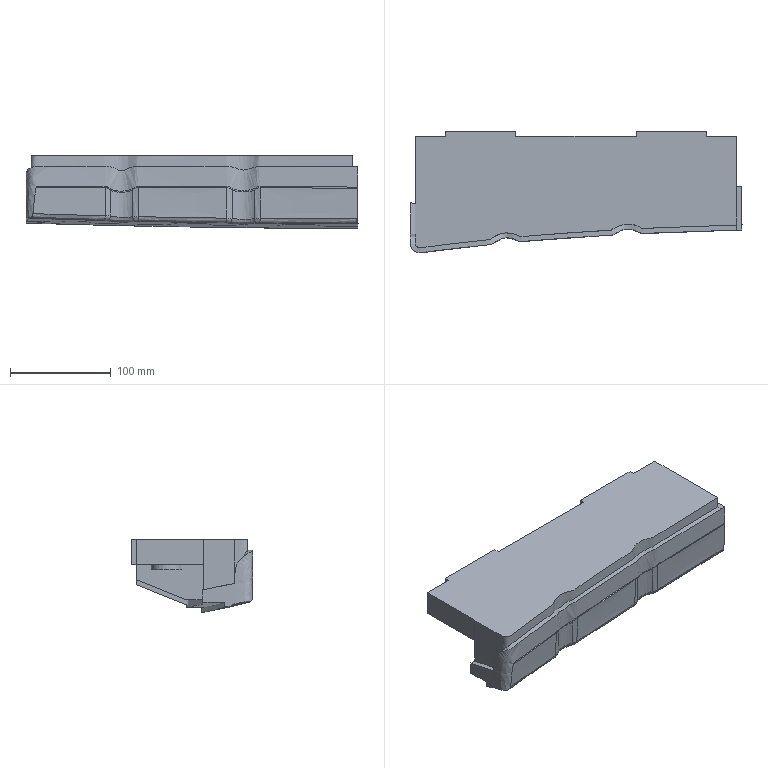Part | NX | features solid 2 | 1 solid | 91 faces | box 330.281 x 120.893 x 72.552 mm | volume 1547230 mm3 | spline 56 | plane 30 | cylinder 5 | commonest cylinder face diameters 30 x5